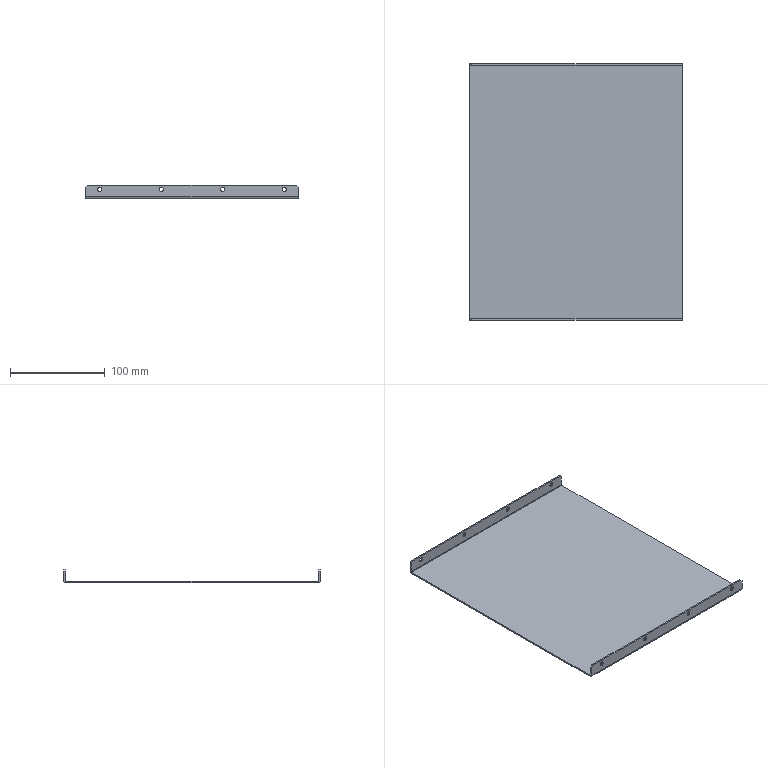Part | STEP file | GLSJ-10-37 | 1 solid | 42 faces | box 225 x 271.5 x 14.5 mm | volume 99773 mm3 | plane 22 | cylinder 20 | commonest cylinder face diameters 4.5 x16 1.473 x2 4.473 x2